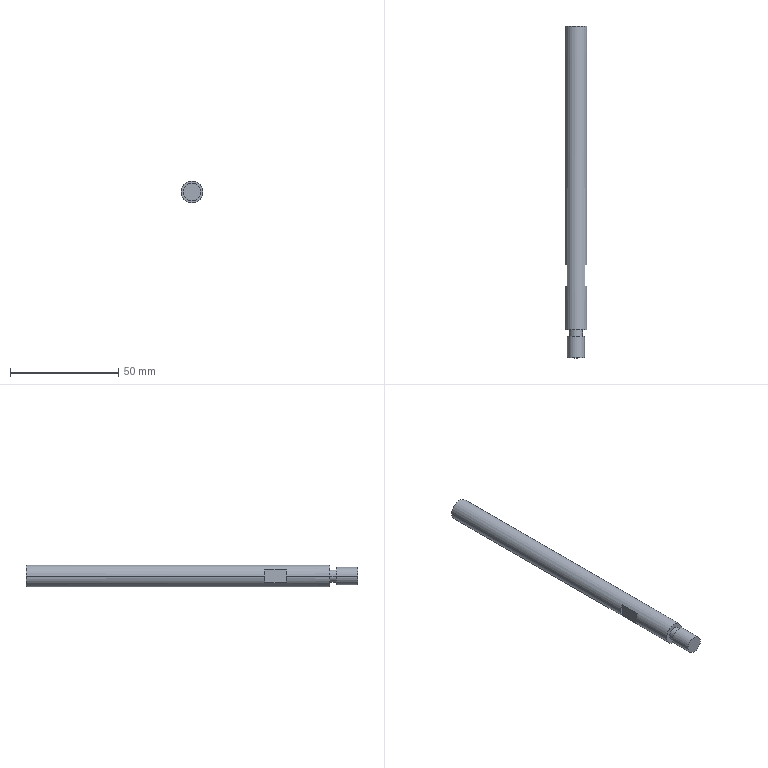Part | SolidWorks | features HoleWzd 1, ICE 1, Revolution 1 | 1 solid | 20 faces | box 10 x 153 x 10 mm | volume 11256 mm3 | plane 10 | cylinder 8 | cone 2 | commonest cylinder face diameters 5 x2 6 x2 8 x2 10 x2
STEP:
#1=CARTESIAN_POINT('',(0.,2.171,-2.5));
#2=VERTEX_POINT('',#1);
#3=CARTESIAN_POINT('',(0.,2.171,2.5));
#4=VERTEX_POINT('',#3);
#5=CARTESIAN_POINT('',(0.,2.171,0.));
#6=DIRECTION('',(0.,1.,0.));
#7=DIRECTION('',(0.,0.,1.));
#8=AXIS2_PLACEMENT_3D('',#5,#6,#7);
#9=CIRCLE('',#8,2.5);
#10=EDGE_CURVE('',#2,#4,#9,.T.);
#11=ORIENTED_EDGE('',*,*,#10,.F.);
#12=CARTESIAN_POINT('',(0.,14.171,-2.5));
#13=VERTEX_POINT('',#12);
#14=CARTESIAN_POINT('',(0.,14.171,-2.5));
#15=DIRECTION('',(0.,1.,0.));
#16=VECTOR('',#15,1000.);
#17=LINE('',#14,#16);
#18=EDGE_CURVE('',#2,#13,#17,.T.);
#19=ORIENTED_EDGE('',*,*,#18,.T.);
#20=CARTESIAN_POINT('',(0.,14.171,2.5));
#21=VERTEX_POINT('',#20);
#22=CARTESIAN_POINT('',(0.,14.171,0.));
#23=DIRECTION('',(0.,1.,0.));
#24=DIRECTION('',(0.,0.,1.));
#25=AXIS2_PLACEMENT_3D('',#22,#23,#24);
#26=CIRCLE('',#25,2.5);
#27=EDGE_CURVE('',#13,#21,#26,.T.);
#28=ORIENTED_EDGE('',*,*,#27,.T.);
#29=CARTESIAN_POINT('',(0.,14.171,2.5));
#30=DIRECTION('',(0.,1.,0.));
#31=VECTOR('',#30,1000.);
#32=LINE('',#29,#31);
#33=EDGE_CURVE('',#4,#21,#32,.T.);
#34=ORIENTED_EDGE('',*,*,#33,.F.);
#35=EDGE_LOOP('',(#11,#19,#28,#34));
#36=FACE_OUTER_BOUND('',#35,.T.);
#37=CARTESIAN_POINT('',(0.,14.171,0.));
#38=DIRECTION('',(0.,1.,0.));
#39=DIRECTION('',(0.,0.,1.));
#40=AXIS2_PLACEMENT_3D('',#37,#38,#39);
#41=CYLINDRICAL_SURFACE('',#40,2.5);
#42=ADVANCED_FACE('',(#36),#41,.F.);
#43=CARTESIAN_POINT('',(0.,0.6688,0.));
#44=VERTEX_POINT('',#43);
#45=CARTESIAN_POINT('',(0.,2.171,2.5));
#46=DIRECTION('',(0.,0.515,0.8572));
#47=VECTOR('',#46,1000.);
#48=LINE('',#45,#47);
#49=EDGE_CURVE('',#44,#4,#48,.T.);
#50=ORIENTED_EDGE('',*,*,#49,.F.);
#51=CARTESIAN_POINT('',(0.,2.171,-2.5));
#52=DIRECTION('',(0.,0.515,-0.8572));
#53=VECTOR('',#52,1000.);
#54=LINE('',#51,#53);
#55=EDGE_CURVE('',#44,#2,#54,.T.);
#56=ORIENTED_EDGE('',*,*,#55,.T.);
#57=ORIENTED_EDGE('',*,*,#10,.T.);
#58=EDGE_LOOP('',(#50,#56,#57));
#59=FACE_OUTER_BOUND('',#58,.T.);
#60=CARTESIAN_POINT('',(0.,2.171,0.));
#61=DIRECTION('',(0.,1.,0.));
#62=DIRECTION('',(0.,0.,1.));
#63=AXIS2_PLACEMENT_3D('',#60,#61,#62);
#64=CONICAL_SURFACE('',#63,2.5,1.03);
#65=ADVANCED_FACE('',(#59),#64,.F.);
#66=CARTESIAN_POINT('',(-5.,-125.829,0.));
#67=VERTEX_POINT('',#66);
#68=CARTESIAN_POINT('',(5.,-125.829,0.));
#69=VERTEX_POINT('',#68);
#70=CARTESIAN_POINT('',(0.,-125.829,0.));
#71=DIRECTION('',(0.,1.,0.));
#72=DIRECTION('',(-1.,0.,0.));
#73=AXIS2_PLACEMENT_3D('',#70,#71,#72);
#74=CIRCLE('',#73,5.);
#75=EDGE_CURVE('',#67,#69,#74,.T.);
#76=ORIENTED_EDGE('',*,*,#75,.T.);
#77=CARTESIAN_POINT('',(5.,-105.829,0.));
#78=VERTEX_POINT('',#77);
#79=CARTESIAN_POINT('',(5.,14.171,0.));
#80=DIRECTION('',(0.,1.,0.));
#81=VECTOR('',#80,1000.);
#82=LINE('',#79,#81);
#83=EDGE_CURVE('',#69,#78,#82,.T.);
#84=ORIENTED_EDGE('',*,*,#83,.T.);
#85=CARTESIAN_POINT('',(4.,-105.829,3.));
#86=VERTEX_POINT('',#85);
#87=CARTESIAN_POINT('',(0.,-105.829,0.));
#88=DIRECTION('',(0.,1.,0.));
#89=DIRECTION('',(0.,0.,-1.));
#90=AXIS2_PLACEMENT_3D('',#87,#88,#89);
#91=CIRCLE('',#90,5.);
#92=EDGE_CURVE('',#86,#78,#91,.T.);
#93=ORIENTED_EDGE('',*,*,#92,.F.);
#94=CARTESIAN_POINT('',(4.,-95.829,3.));
#95=VERTEX_POINT('',#94);
#96=CARTESIAN_POINT('',(4.,14.171,3.));
#97=DIRECTION('',(0.,-1.,0.));
#98=VECTOR('',#97,1000.);
#99=LINE('',#96,#98);
#100=EDGE_CURVE('',#95,#86,#99,.T.);
#101=ORIENTED_EDGE('',*,*,#100,.F.);
#102=CARTESIAN_POINT('',(5.,-95.829,0.));
#103=VERTEX_POINT('',#102);
#104=CARTESIAN_POINT('',(0.,-95.829,0.));
#105=DIRECTION('',(0.,-1.,0.));
#106=DIRECTION('',(0.,0.,1.));
#107=AXIS2_PLACEMENT_3D('',#104,#105,#106);
#108=CIRCLE('',#107,5.);
#109=EDGE_CURVE('',#103,#95,#108,.T.);
#110=ORIENTED_EDGE('',*,*,#109,.F.);
#111=CARTESIAN_POINT('',(5.,14.171,0.));
#112=VERTEX_POINT('',#111);
#113=CARTESIAN_POINT('',(5.,14.171,0.));
#114=DIRECTION('',(0.,1.,0.));
#115=VECTOR('',#114,1000.);
#116=LINE('',#113,#115);
#117=EDGE_CURVE('',#103,#112,#116,.T.);
#118=ORIENTED_EDGE('',*,*,#117,.T.);
#119=CARTESIAN_POINT('',(-5.,14.171,0.));
#120=VERTEX_POINT('',#119);
#121=CARTESIAN_POINT('',(0.,14.171,0.));
#122=DIRECTION('',(0.,1.,0.));
#123=DIRECTION('',(-1.,0.,0.));
#124=AXIS2_PLACEMENT_3D('',#121,#122,#123);
#125=CIRCLE('',#124,5.);
#126=EDGE_CURVE('',#120,#112,#125,.T.);
#127=ORIENTED_EDGE('',*,*,#126,.F.);
#128=CARTESIAN_POINT('',(-5.,-95.829,0.));
#129=VERTEX_POINT('',#128);
#130=CARTESIAN_POINT('',(-5.,14.171,0.));
#131=DIRECTION('',(0.,1.,0.));
#132=VECTOR('',#131,1000.);
#133=LINE('',#130,#132);
#134=EDGE_CURVE('',#129,#120,#133,.T.);
#135=ORIENTED_EDGE('',*,*,#134,.F.);
#136=CARTESIAN_POINT('',(-4.,-95.829,3.));
#137=VERTEX_POINT('',#136);
#138=CARTESIAN_POINT('',(0.,-95.829,0.));
#139=DIRECTION('',(0.,-1.,0.));
#140=DIRECTION('',(0.,0.,1.));
#141=AXIS2_PLACEMENT_3D('',#138,#139,#140);
#142=CIRCLE('',#141,5.);
#143=EDGE_CURVE('',#137,#129,#142,.T.);
#144=ORIENTED_EDGE('',*,*,#143,.F.);
#145=CARTESIAN_POINT('',(-4.,-105.829,3.));
#146=VERTEX_POINT('',#145);
#147=CARTESIAN_POINT('',(-4.,14.171,3.));
#148=DIRECTION('',(0.,1.,0.));
#149=VECTOR('',#148,1000.);
#150=LINE('',#147,#149);
#151=EDGE_CURVE('',#146,#137,#150,.T.);
#152=ORIENTED_EDGE('',*,*,#151,.F.);
#153=CARTESIAN_POINT('',(-5.,-105.829,0.));
#154=VERTEX_POINT('',#153);
#155=CARTESIAN_POINT('',(0.,-105.829,0.));
#156=DIRECTION('',(0.,1.,0.));
#157=DIRECTION('',(0.,0.,-1.));
#158=AXIS2_PLACEMENT_3D('',#155,#156,#157);
#159=CIRCLE('',#158,5.);
#160=EDGE_CURVE('',#154,#146,#159,.T.);
#161=ORIENTED_EDGE('',*,*,#160,.F.);
#162=CARTESIAN_POINT('',(-5.,14.171,0.));
#163=DIRECTION('',(0.,1.,0.));
#164=VECTOR('',#163,1000.);
#165=LINE('',#162,#164);
#166=EDGE_CURVE('',#67,#154,#165,.T.);
#167=ORIENTED_EDGE('',*,*,#166,.F.);
#168=EDGE_LOOP('',(#76,#84,#93,#101,#110,#118,#127,#135,#144,#152,#161,#167));
#169=FACE_OUTER_BOUND('',#168,.T.);
#170=CARTESIAN_POINT('',(0.,14.171,0.));
#171=DIRECTION('',(0.,1.,0.));
#172=DIRECTION('',(-1.,0.,0.));
#173=AXIS2_PLACEMENT_3D('',#170,#171,#172);
#174=CYLINDRICAL_SURFACE('',#173,5.);
#175=ADVANCED_FACE('',(#169),#174,.T.);
#176=CARTESIAN_POINT('',(-3.,-128.829,0.));
#177=VERTEX_POINT('',#176);
#178=CARTESIAN_POINT('',(3.,-128.829,0.));
#179=VERTEX_POINT('',#178);
#180=CARTESIAN_POINT('',(0.,-128.829,0.));
#181=DIRECTION('',(0.,1.,0.));
#182=DIRECTION('',(-1.,0.,0.));
#183=AXIS2_PLACEMENT_3D('',#180,#181,#182);
#184=CIRCLE('',#183,3.);
#185=EDGE_CURVE('',#177,#179,#184,.T.);
#186=ORIENTED_EDGE('',*,*,#185,.T.);
#187=CARTESIAN_POINT('',(3.,-125.829,0.));
#188=VERTEX_POINT('',#187);
#189=CARTESIAN_POINT('',(3.,14.171,0.));
#190=DIRECTION('',(0.,1.,0.));
#191=VECTOR('',#190,1000.);
#192=LINE('',#189,#191);
#193=EDGE_CURVE('',#179,#188,#192,.T.);
#194=ORIENTED_EDGE('',*,*,#193,.T.);
#195=CARTESIAN_POINT('',(-3.,-125.829,0.));
#196=VERTEX_POINT('',#195);
#197=CARTESIAN_POINT('',(0.,-125.829,0.));
#198=DIRECTION('',(0.,1.,0.));
#199=DIRECTION('',(-1.,0.,0.));
#200=AXIS2_PLACEMENT_3D('',#197,#198,#199);
#201=CIRCLE('',#200,3.);
#202=EDGE_CURVE('',#196,#188,#201,.T.);
#203=ORIENTED_EDGE('',*,*,#202,.F.);
#204=CARTESIAN_POINT('',(-3.,14.171,0.));
#205=DIRECTION('',(0.,1.,0.));
#206=VECTOR('',#205,1000.);
#207=LINE('',#204,#206);
#208=EDGE_CURVE('',#177,#196,#207,.T.);
#209=ORIENTED_EDGE('',*,*,#208,.F.);
#210=EDGE_LOOP('',(#186,#194,#203,#209));
#211=FACE_OUTER_BOUND('',#210,.T.);
#212=CARTESIAN_POINT('',(0.,14.171,0.));
#213=DIRECTION('',(0.,1.,0.));
#214=DIRECTION('',(-1.,0.,0.));
#215=AXIS2_PLACEMENT_3D('',#212,#213,#214);
#216=CYLINDRICAL_SURFACE('',#215,3.);
#217=ADVANCED_FACE('',(#211),#216,.T.);
#218=CARTESIAN_POINT('',(-4.,-138.829,0.));
#219=VERTEX_POINT('',#218);
#220=CARTESIAN_POINT('',(4.,-138.829,0.));
#221=VERTEX_POINT('',#220);
#222=CARTESIAN_POINT('',(0.,-138.829,0.));
#223=DIRECTION('',(0.,1.,0.));
#224=DIRECTION('',(-1.,0.,0.));
#225=AXIS2_PLACEMENT_3D('',#222,#223,#224);
#226=CIRCLE('',#225,4.);
#227=EDGE_CURVE('',#219,#221,#226,.T.);
#228=ORIENTED_EDGE('',*,*,#227,.T.);
#229=CARTESIAN_POINT('',(4.,-128.829,0.));
#230=VERTEX_POINT('',#229);
#231=CARTESIAN_POINT('',(4.,14.171,0.));
#232=DIRECTION('',(0.,1.,0.));
#233=VECTOR('',#232,1000.);
#234=LINE('',#231,#233);
#235=EDGE_CURVE('',#221,#230,#234,.T.);
#236=ORIENTED_EDGE('',*,*,#235,.T.);
#237=CARTESIAN_POINT('',(-4.,-128.829,0.));
#238=VERTEX_POINT('',#237);
#239=CARTESIAN_POINT('',(0.,-128.829,0.));
#240=DIRECTION('',(0.,1.,0.));
#241=DIRECTION('',(-1.,0.,0.));
#242=AXIS2_PLACEMENT_3D('',#239,#240,#241);
#243=CIRCLE('',#242,4.);
#244=EDGE_CURVE('',#238,#230,#243,.T.);
#245=ORIENTED_EDGE('',*,*,#244,.F.);
#246=CARTESIAN_POINT('',(-4.,14.171,0.));
#247=DIRECTION('',(0.,1.,0.));
#248=VECTOR('',#247,1000.);
#249=LINE('',#246,#248);
#250=EDGE_CURVE('',#219,#238,#249,.T.);
#251=ORIENTED_EDGE('',*,*,#250,.F.);
#252=EDGE_LOOP('',(#228,#236,#245,#251));
#253=FACE_OUTER_BOUND('',#252,.T.);
#254=CARTESIAN_POINT('',(0.,14.171,0.));
#255=DIRECTION('',(0.,1.,0.));
#256=DIRECTION('',(-1.,0.,0.));
#257=AXIS2_PLACEMENT_3D('',#254,#255,#256);
#258=CYLINDRICAL_SURFACE('',#257,4.);
#259=ADVANCED_FACE('',(#253),#258,.T.);
#260=CARTESIAN_POINT('',(0.,14.171,0.));
#261=DIRECTION('',(0.,1.,0.));
#262=DIRECTION('',(0.,0.,1.));
#263=AXIS2_PLACEMENT_3D('',#260,#261,#262);
#264=CIRCLE('',#263,2.5);
#265=EDGE_CURVE('',#21,#13,#264,.T.);
#266=ORIENTED_EDGE('',*,*,#265,.F.);
#267=ORIENTED_EDGE('',*,*,#27,.F.);
#268=EDGE_LOOP('',(#266,#267));
#269=FACE_BOUND('',#268,.T.);
#270=ORIENTED_EDGE('',*,*,#126,.T.);
#271=CARTESIAN_POINT('',(0.,14.171,0.));
#272=DIRECTION('',(0.,1.,0.));
#273=DIRECTION('',(-1.,0.,0.));
#274=AXIS2_PLACEMENT_3D('',#271,#272,#273);
#275=CIRCLE('',#274,5.);
#276=EDGE_CURVE('',#112,#120,#275,.T.);
#277=ORIENTED_EDGE('',*,*,#276,.T.);
#278=EDGE_LOOP('',(#270,#277));
#279=FACE_OUTER_BOUND('',#278,.T.);
#280=CARTESIAN_POINT('',(-5.,14.171,0.));
#281=DIRECTION('',(0.,1.,0.));
#282=DIRECTION('',(-1.,0.,0.));
#283=AXIS2_PLACEMENT_3D('',#280,#281,#282);
#284=PLANE('',#283);
#285=ADVANCED_FACE('',(#269,#279),#284,.T.);
#286=ORIENTED_EDGE('',*,*,#227,.F.);
#287=CARTESIAN_POINT('',(0.,-138.829,0.));
#288=DIRECTION('',(0.,1.,0.));
#289=DIRECTION('',(-1.,0.,0.));
#290=AXIS2_PLACEMENT_3D('',#287,#288,#289);
#291=CIRCLE('',#290,4.);
#292=EDGE_CURVE('',#221,#219,#291,.T.);
#293=ORIENTED_EDGE('',*,*,#292,.F.);
#294=EDGE_LOOP('',(#286,#293));
#295=FACE_OUTER_BOUND('',#294,.T.);
#296=CARTESIAN_POINT('',(0.,-138.829,0.));
#297=DIRECTION('',(0.,-1.,0.));
#298=DIRECTION('',(1.,0.,0.));
#299=AXIS2_PLACEMENT_3D('',#296,#297,#298);
#300=PLANE('',#299);
#301=ADVANCED_FACE('',(#295),#300,.T.);
#302=ORIENTED_EDGE('',*,*,#235,.F.);
#303=ORIENTED_EDGE('',*,*,#292,.T.);
#304=ORIENTED_EDGE('',*,*,#250,.T.);
#305=CARTESIAN_POINT('',(0.,-128.829,0.));
#306=DIRECTION('',(0.,1.,0.));
#307=DIRECTION('',(-1.,0.,0.));
#308=AXIS2_PLACEMENT_3D('',#305,#306,#307);
#309=CIRCLE('',#308,4.);
#310=EDGE_CURVE('',#230,#238,#309,.T.);
#311=ORIENTED_EDGE('',*,*,#310,.F.);
#312=EDGE_LOOP('',(#302,#303,#304,#311));
#313=FACE_OUTER_BOUND('',#312,.T.);
#314=CARTESIAN_POINT('',(0.,14.171,0.));
#315=DIRECTION('',(0.,1.,0.));
#316=DIRECTION('',(-1.,0.,0.));
#317=AXIS2_PLACEMENT_3D('',#314,#315,#316);
#318=CYLINDRICAL_SURFACE('',#317,4.);
#319=ADVANCED_FACE('',(#313),#318,.T.);
#320=ORIENTED_EDGE('',*,*,#244,.T.);
#321=ORIENTED_EDGE('',*,*,#310,.T.);
#322=EDGE_LOOP('',(#320,#321));
#323=FACE_OUTER_BOUND('',#322,.T.);
#324=ORIENTED_EDGE('',*,*,#185,.F.);
#325=CARTESIAN_POINT('',(0.,-128.829,0.));
#326=DIRECTION('',(0.,1.,0.));
#327=DIRECTION('',(-1.,0.,0.));
#328=AXIS2_PLACEMENT_3D('',#325,#326,#327);
#329=CIRCLE('',#328,3.);
#330=EDGE_CURVE('',#179,#177,#329,.T.);
#331=ORIENTED_EDGE('',*,*,#330,.F.);
#332=EDGE_LOOP('',(#324,#331));
#333=FACE_BOUND('',#332,.T.);
#334=CARTESIAN_POINT('',(-4.,-128.829,0.));
#335=DIRECTION('',(0.,1.,0.));
#336=DIRECTION('',(-1.,0.,0.));
#337=AXIS2_PLACEMENT_3D('',#334,#335,#336);
#338=PLANE('',#337);
#339=ADVANCED_FACE('',(#323,#333),#338,.T.);
#340=ORIENTED_EDGE('',*,*,#193,.F.);
#341=ORIENTED_EDGE('',*,*,#330,.T.);
#342=ORIENTED_EDGE('',*,*,#208,.T.);
#343=CARTESIAN_POINT('',(0.,-125.829,0.));
#344=DIRECTION('',(0.,1.,0.));
#345=DIRECTION('',(-1.,0.,0.));
#346=AXIS2_PLACEMENT_3D('',#343,#344,#345);
#347=CIRCLE('',#346,3.);
#348=EDGE_CURVE('',#188,#196,#347,.T.);
#349=ORIENTED_EDGE('',*,*,#348,.F.);
#350=EDGE_LOOP('',(#340,#341,#342,#349));
#351=FACE_OUTER_BOUND('',#350,.T.);
#352=CARTESIAN_POINT('',(0.,14.171,0.));
#353=DIRECTION('',(0.,1.,0.));
#354=DIRECTION('',(-1.,0.,0.));
#355=AXIS2_PLACEMENT_3D('',#352,#353,#354);
#356=CYLINDRICAL_SURFACE('',#355,3.);
#357=ADVANCED_FACE('',(#351),#356,.T.);
#358=ORIENTED_EDGE('',*,*,#202,.T.);
#359=ORIENTED_EDGE('',*,*,#348,.T.);
#360=EDGE_LOOP('',(#358,#359));
#361=FACE_BOUND('',#360,.T.);
#362=ORIENTED_EDGE('',*,*,#75,.F.);
#363=CARTESIAN_POINT('',(0.,-125.829,0.));
#364=DIRECTION('',(0.,1.,0.));
#365=DIRECTION('',(-1.,0.,0.));
#366=AXIS2_PLACEMENT_3D('',#363,#364,#365);
#367=CIRCLE('',#366,5.);
#368=EDGE_CURVE('',#69,#67,#367,.T.);
#369=ORIENTED_EDGE('',*,*,#368,.F.);
#370=EDGE_LOOP('',(#362,#369));
#371=FACE_OUTER_BOUND('',#370,.T.);
#372=CARTESIAN_POINT('',(-3.,-125.829,0.));
#373=DIRECTION('',(0.,-1.,0.));
#374=DIRECTION('',(1.,0.,0.));
#375=AXIS2_PLACEMENT_3D('',#372,#373,#374);
#376=PLANE('',#375);
#377=ADVANCED_FACE('',(#361,#371),#376,.T.);
#378=ORIENTED_EDGE('',*,*,#83,.F.);
#379=ORIENTED_EDGE('',*,*,#368,.T.);
#380=ORIENTED_EDGE('',*,*,#166,.T.);
#381=CARTESIAN_POINT('',(-4.,-105.829,-3.));
#382=VERTEX_POINT('',#381);
#383=CARTESIAN_POINT('',(0.,-105.829,0.));
#384=DIRECTION('',(0.,1.,0.));
#385=DIRECTION('',(0.,0.,-1.));
#386=AXIS2_PLACEMENT_3D('',#383,#384,#385);
#387=CIRCLE('',#386,5.);
#388=EDGE_CURVE('',#382,#154,#387,.T.);
#389=ORIENTED_EDGE('',*,*,#388,.F.);
#390=CARTESIAN_POINT('',(-4.,-95.829,-3.));
#391=VERTEX_POINT('',#390);
#392=CARTESIAN_POINT('',(-4.,14.171,-3.));
#393=DIRECTION('',(0.,-1.,0.));
#394=VECTOR('',#393,1000.);
#395=LINE('',#392,#394);
#396=EDGE_CURVE('',#391,#382,#395,.T.);
#397=ORIENTED_EDGE('',*,*,#396,.F.);
#398=CARTESIAN_POINT('',(0.,-95.829,0.));
#399=DIRECTION('',(0.,-1.,0.));
#400=DIRECTION('',(0.,0.,1.));
#401=AXIS2_PLACEMENT_3D('',#398,#399,#400);
#402=CIRCLE('',#401,5.);
#403=EDGE_CURVE('',#129,#391,#402,.T.);
#404=ORIENTED_EDGE('',*,*,#403,.F.);
#405=ORIENTED_EDGE('',*,*,#134,.T.);
#406=ORIENTED_EDGE('',*,*,#276,.F.);
#407=ORIENTED_EDGE('',*,*,#117,.F.);
#408=CARTESIAN_POINT('',(4.,-95.829,-3.));
#409=VERTEX_POINT('',#408);
#410=CARTESIAN_POINT('',(0.,-95.829,0.));
#411=DIRECTION('',(0.,-1.,0.));
#412=DIRECTION('',(0.,0.,1.));
#413=AXIS2_PLACEMENT_3D('',#410,#411,#412);
#414=CIRCLE('',#413,5.);
#415=EDGE_CURVE('',#409,#103,#414,.T.);
#416=ORIENTED_EDGE('',*,*,#415,.F.);
#417=CARTESIAN_POINT('',(4.,-105.829,-3.));
#418=VERTEX_POINT('',#417);
#419=CARTESIAN_POINT('',(4.,14.171,-3.));
#420=DIRECTION('',(0.,1.,0.));
#421=VECTOR('',#420,1000.);
#422=LINE('',#419,#421);
#423=EDGE_CURVE('',#418,#409,#422,.T.);
#424=ORIENTED_EDGE('',*,*,#423,.F.);
#425=CARTESIAN_POINT('',(0.,-105.829,0.));
#426=DIRECTION('',(0.,1.,0.));
#427=DIRECTION('',(0.,0.,-1.));
#428=AXIS2_PLACEMENT_3D('',#425,#426,#427);
#429=CIRCLE('',#428,5.);
#430=EDGE_CURVE('',#78,#418,#429,.T.);
#431=ORIENTED_EDGE('',*,*,#430,.F.);
#432=EDGE_LOOP('',(#378,#379,#380,#389,#397,#404,#405,#406,#407,#416,#424,#431));
#433=FACE_OUTER_BOUND('',#432,.T.);
#434=CARTESIAN_POINT('',(0.,14.171,0.));
#435=DIRECTION('',(0.,1.,0.));
#436=DIRECTION('',(-1.,0.,0.));
#437=AXIS2_PLACEMENT_3D('',#434,#435,#436);
#438=CYLINDRICAL_SURFACE('',#437,5.);
#439=ADVANCED_FACE('',(#433),#438,.T.);
#440=ORIENTED_EDGE('',*,*,#415,.T.);
#441=ORIENTED_EDGE('',*,*,#109,.T.);
#442=CARTESIAN_POINT('',(4.,-95.829,-5.));
#443=DIRECTION('',(0.,0.,1.));
#444=VECTOR('',#443,1000.);
#445=LINE('',#442,#444);
#446=EDGE_CURVE('',#409,#95,#445,.T.);
#447=ORIENTED_EDGE('',*,*,#446,.F.);
#448=EDGE_LOOP('',(#440,#441,#447));
#449=FACE_OUTER_BOUND('',#448,.T.);
#450=CARTESIAN_POINT('',(5.,-95.829,-5.));
#451=DIRECTION('',(0.,1.,0.));
#452=DIRECTION('',(0.,0.,1.));
#453=AXIS2_PLACEMENT_3D('',#450,#451,#452);
#454=PLANE('',#453);
#455=ADVANCED_FACE('',(#449),#454,.F.);
#456=CARTESIAN_POINT('',(4.,-105.829,-5.));
#457=DIRECTION('',(0.,0.,1.));
#458=VECTOR('',#457,1000.);
#459=LINE('',#456,#458);
#460=EDGE_CURVE('',#418,#86,#459,.T.);
#461=ORIENTED_EDGE('',*,*,#460,.T.);
#462=ORIENTED_EDGE('',*,*,#92,.T.);
#463=ORIENTED_EDGE('',*,*,#430,.T.);
#464=EDGE_LOOP('',(#461,#462,#463));
#465=FACE_OUTER_BOUND('',#464,.T.);
#466=CARTESIAN_POINT('',(5.,-105.829,-5.));
#467=DIRECTION('',(0.,-1.,0.));
#468=DIRECTION('',(0.,0.,-1.));
#469=AXIS2_PLACEMENT_3D('',#466,#467,#468);
#470=PLANE('',#469);
#471=ADVANCED_FACE('',(#465),#470,.F.);
#472=ORIENTED_EDGE('',*,*,#100,.T.);
#473=ORIENTED_EDGE('',*,*,#460,.F.);
#474=ORIENTED_EDGE('',*,*,#423,.T.);
#475=ORIENTED_EDGE('',*,*,#446,.T.);
#476=EDGE_LOOP('',(#472,#473,#474,#475));
#477=FACE_OUTER_BOUND('',#476,.T.);
#478=CARTESIAN_POINT('',(4.,-95.829,-5.));
#479=DIRECTION('',(-1.,0.,0.));
#480=DIRECTION('',(0.,-1.,0.));
#481=AXIS2_PLACEMENT_3D('',#478,#479,#480);
#482=PLANE('',#481);
#483=ADVANCED_FACE('',(#477),#482,.F.);
#484=CARTESIAN_POINT('',(-4.,-95.829,-5.));
#485=DIRECTION('',(0.,0.,1.));
#486=VECTOR('',#485,1000.);
#487=LINE('',#484,#486);
#488=EDGE_CURVE('',#391,#137,#487,.T.);
#489=ORIENTED_EDGE('',*,*,#488,.T.);
#490=ORIENTED_EDGE('',*,*,#143,.T.);
#491=ORIENTED_EDGE('',*,*,#403,.T.);
#492=EDGE_LOOP('',(#489,#490,#491));
#493=FACE_OUTER_BOUND('',#492,.T.);
#494=CARTESIAN_POINT('',(-5.,-95.829,-5.));
#495=DIRECTION('',(0.,1.,0.));
#496=DIRECTION('',(0.,0.,1.));
#497=AXIS2_PLACEMENT_3D('',#494,#495,#496);
#498=PLANE('',#497);
#499=ADVANCED_FACE('',(#493),#498,.F.);
#500=ORIENTED_EDGE('',*,*,#396,.T.);
#501=CARTESIAN_POINT('',(-4.,-105.829,-5.));
#502=DIRECTION('',(0.,0.,1.));
#503=VECTOR('',#502,1000.);
#504=LINE('',#501,#503);
#505=EDGE_CURVE('',#382,#146,#504,.T.);
#506=ORIENTED_EDGE('',*,*,#505,.T.);
#507=ORIENTED_EDGE('',*,*,#151,.T.);
#508=ORIENTED_EDGE('',*,*,#488,.F.);
#509=EDGE_LOOP('',(#500,#506,#507,#508));
#510=FACE_OUTER_BOUND('',#509,.T.);
#511=CARTESIAN_POINT('',(-4.,-95.829,-5.));
#512=DIRECTION('',(1.,0.,0.));
#513=DIRECTION('',(0.,1.,0.));
#514=AXIS2_PLACEMENT_3D('',#511,#512,#513);
#515=PLANE('',#514);
#516=ADVANCED_FACE('',(#510),#515,.F.);
#517=ORIENTED_EDGE('',*,*,#505,.F.);
#518=ORIENTED_EDGE('',*,*,#388,.T.);
#519=ORIENTED_EDGE('',*,*,#160,.T.);
#520=EDGE_LOOP('',(#517,#518,#519));
#521=FACE_OUTER_BOUND('',#520,.T.);
#522=CARTESIAN_POINT('',(-5.,-105.829,-5.));
#523=DIRECTION('',(0.,-1.,0.));
#524=DIRECTION('',(0.,0.,-1.));
#525=AXIS2_PLACEMENT_3D('',#522,#523,#524);
#526=PLANE('',#525);
#527=ADVANCED_FACE('',(#521),#526,.F.);
#528=ORIENTED_EDGE('',*,*,#55,.F.);
#529=ORIENTED_EDGE('',*,*,#49,.T.);
#530=CARTESIAN_POINT('',(0.,2.171,0.));
#531=DIRECTION('',(0.,1.,0.));
#532=DIRECTION('',(0.,0.,1.));
#533=AXIS2_PLACEMENT_3D('',#530,#531,#532);
#534=CIRCLE('',#533,2.5);
#535=EDGE_CURVE('',#4,#2,#534,.T.);
#536=ORIENTED_EDGE('',*,*,#535,.T.);
#537=EDGE_LOOP('',(#528,#529,#536));
#538=FACE_OUTER_BOUND('',#537,.T.);
#539=CARTESIAN_POINT('',(0.,2.171,0.));
#540=DIRECTION('',(0.,1.,0.));
#541=DIRECTION('',(0.,0.,1.));
#542=AXIS2_PLACEMENT_3D('',#539,#540,#541);
#543=CONICAL_SURFACE('',#542,2.5,1.03);
#544=ADVANCED_FACE('',(#538),#543,.F.);
#545=ORIENTED_EDGE('',*,*,#18,.F.);
#546=ORIENTED_EDGE('',*,*,#535,.F.);
#547=ORIENTED_EDGE('',*,*,#33,.T.);
#548=ORIENTED_EDGE('',*,*,#265,.T.);
#549=EDGE_LOOP('',(#545,#546,#547,#548));
#550=FACE_OUTER_BOUND('',#549,.T.);
#551=CARTESIAN_POINT('',(0.,14.171,0.));
#552=DIRECTION('',(0.,1.,0.));
#553=DIRECTION('',(0.,0.,1.));
#554=AXIS2_PLACEMENT_3D('',#551,#552,#553);
#555=CYLINDRICAL_SURFACE('',#554,2.5);
#556=ADVANCED_FACE('',(#550),#555,.F.);
#557=CLOSED_SHELL('',(#42,#65,#175,#217,#259,#285,#301,#319,#339,#357,#377,#439,#455,#471,#483,#499,#516,#527,#544,#556));
#558=MANIFOLD_SOLID_BREP('',#557);
#559=CARTESIAN_POINT('',(0.,0.,0.));
#560=DIRECTION('',(0.,0.,1.));
#561=DIRECTION('',(1.,0.,0.));
#562=AXIS2_PLACEMENT_3D('',#559,#560,#561);
#563=(LENGTH_UNIT()NAMED_UNIT(*)SI_UNIT(.MILLI.,.METRE.));
#564=UNCERTAINTY_MEASURE_WITH_UNIT(LENGTH_MEASURE(0.00001),#563,'','');
#565=(NAMED_UNIT(*)PLANE_ANGLE_UNIT()SI_UNIT($,.RADIAN.));
#566=(NAMED_UNIT(*)SI_UNIT($,.STERADIAN.)SOLID_ANGLE_UNIT());
#567=(GEOMETRIC_REPRESENTATION_CONTEXT(3)GLOBAL_UNCERTAINTY_ASSIGNED_CONTEXT((#564))GLOBAL_UNIT_ASSIGNED_CONTEXT((#563,#565,#566))REPRESENTATION_CONTEXT('',''));
#568=ADVANCED_BREP_SHAPE_REPRESENTATION('',(#558,#562),#567);